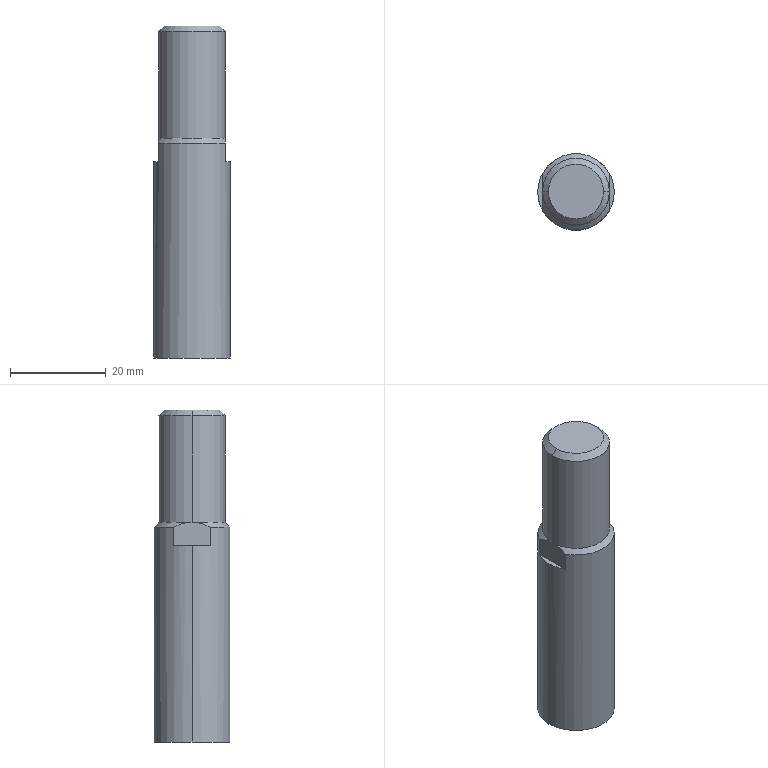Part | STEP file | rA_CDQ2B40_40DM_M9N_0_ | 1 solid | 14 faces | box 16 x 16 x 69.5 mm | volume 12766 mm3 | plane 6 | cylinder 4 | cone 4 | commonest cylinder face diameters 14 x2 16 x2
STEP:
#1=CARTESIAN_POINT('',(8.,0.,-41.));
#2=VERTEX_POINT('',#1);
#3=CARTESIAN_POINT('',(-8.,0.,-41.));
#4=VERTEX_POINT('',#3);
#5=CARTESIAN_POINT('',(0.,0.,-41.));
#6=DIRECTION('',(0.,0.,1.));
#7=DIRECTION('',(1.,0.,0.));
#8=AXIS2_PLACEMENT_3D('',#5,#6,#7);
#9=CIRCLE('',#8,8.);
#10=EDGE_CURVE('',#2,#4,#9,.T.);
#11=ORIENTED_EDGE('',*,*,#10,.T.);
#12=CARTESIAN_POINT('',(-8.,0.,0.1));
#13=VERTEX_POINT('',#12);
#14=CARTESIAN_POINT('',(-8.,0.,-41.));
#15=DIRECTION('',(0.,0.,1.));
#16=VECTOR('',#15,1000.);
#17=LINE('',#14,#16);
#18=EDGE_CURVE('',#4,#13,#17,.T.);
#19=ORIENTED_EDGE('',*,*,#18,.T.);
#20=CARTESIAN_POINT('',(-7.,3.873,0.1));
#21=VERTEX_POINT('',#20);
#22=CARTESIAN_POINT('',(0.,0.,0.1));
#23=DIRECTION('',(0.,0.,1.));
#24=DIRECTION('',(1.,0.,0.));
#25=AXIS2_PLACEMENT_3D('',#22,#23,#24);
#26=CIRCLE('',#25,8.);
#27=EDGE_CURVE('',#21,#13,#26,.T.);
#28=ORIENTED_EDGE('',*,*,#27,.F.);
#29=CARTESIAN_POINT('',(-7.,3.873,4.));
#30=VERTEX_POINT('',#29);
#31=CARTESIAN_POINT('',(-7.,3.873,-41.));
#32=DIRECTION('',(0.,0.,1.));
#33=VECTOR('',#32,1000.);
#34=LINE('',#31,#33);
#35=EDGE_CURVE('',#21,#30,#34,.T.);
#36=ORIENTED_EDGE('',*,*,#35,.T.);
#37=CARTESIAN_POINT('',(7.,3.873,4.));
#38=VERTEX_POINT('',#37);
#39=CARTESIAN_POINT('',(0.,0.,4.));
#40=DIRECTION('',(0.,0.,1.));
#41=DIRECTION('',(1.,0.,0.));
#42=AXIS2_PLACEMENT_3D('',#39,#40,#41);
#43=CIRCLE('',#42,8.);
#44=EDGE_CURVE('',#38,#30,#43,.T.);
#45=ORIENTED_EDGE('',*,*,#44,.F.);
#46=CARTESIAN_POINT('',(7.,3.873,0.1));
#47=VERTEX_POINT('',#46);
#48=CARTESIAN_POINT('',(7.,3.873,-41.));
#49=DIRECTION('',(0.,0.,-1.));
#50=VECTOR('',#49,1000.);
#51=LINE('',#48,#50);
#52=EDGE_CURVE('',#38,#47,#51,.T.);
#53=ORIENTED_EDGE('',*,*,#52,.T.);
#54=CARTESIAN_POINT('',(8.,0.,0.1));
#55=VERTEX_POINT('',#54);
#56=CARTESIAN_POINT('',(0.,0.,0.1));
#57=DIRECTION('',(0.,0.,1.));
#58=DIRECTION('',(1.,0.,0.));
#59=AXIS2_PLACEMENT_3D('',#56,#57,#58);
#60=CIRCLE('',#59,8.);
#61=EDGE_CURVE('',#55,#47,#60,.T.);
#62=ORIENTED_EDGE('',*,*,#61,.F.);
#63=CARTESIAN_POINT('',(8.,0.,-41.));
#64=DIRECTION('',(0.,0.,1.));
#65=VECTOR('',#64,1000.);
#66=LINE('',#63,#65);
#67=EDGE_CURVE('',#2,#55,#66,.T.);
#68=ORIENTED_EDGE('',*,*,#67,.F.);
#69=EDGE_LOOP('',(#11,#19,#28,#36,#45,#53,#62,#68));
#70=FACE_OUTER_BOUND('',#69,.T.);
#71=CARTESIAN_POINT('',(0.,0.,-41.));
#72=DIRECTION('',(0.,0.,1.));
#73=DIRECTION('',(1.,0.,0.));
#74=AXIS2_PLACEMENT_3D('',#71,#72,#73);
#75=CYLINDRICAL_SURFACE('',#74,8.);
#76=ADVANCED_FACE('',(#70),#75,.T.);
#77=CARTESIAN_POINT('',(7.,0.,5.));
#78=VERTEX_POINT('',#77);
#79=CARTESIAN_POINT('',(-7.,0.,5.));
#80=VERTEX_POINT('',#79);
#81=CARTESIAN_POINT('',(0.,0.,5.));
#82=DIRECTION('',(0.,0.,1.));
#83=DIRECTION('',(1.,0.,0.));
#84=AXIS2_PLACEMENT_3D('',#81,#82,#83);
#85=CIRCLE('',#84,7.);
#86=EDGE_CURVE('',#78,#80,#85,.T.);
#87=ORIENTED_EDGE('',*,*,#86,.T.);
#88=CARTESIAN_POINT('',(-7.,0.,27.275));
#89=VERTEX_POINT('',#88);
#90=CARTESIAN_POINT('',(-7.,0.,-41.));
#91=DIRECTION('',(0.,0.,1.));
#92=VECTOR('',#91,1000.);
#93=LINE('',#90,#92);
#94=EDGE_CURVE('',#80,#89,#93,.T.);
#95=ORIENTED_EDGE('',*,*,#94,.T.);
#96=CARTESIAN_POINT('',(7.,0.,27.275));
#97=VERTEX_POINT('',#96);
#98=CARTESIAN_POINT('',(0.,0.,27.275));
#99=DIRECTION('',(0.,0.,1.));
#100=DIRECTION('',(1.,0.,0.));
#101=AXIS2_PLACEMENT_3D('',#98,#99,#100);
#102=CIRCLE('',#101,7.);
#103=EDGE_CURVE('',#97,#89,#102,.T.);
#104=ORIENTED_EDGE('',*,*,#103,.F.);
#105=CARTESIAN_POINT('',(7.,0.,-41.));
#106=DIRECTION('',(0.,0.,1.));
#107=VECTOR('',#106,1000.);
#108=LINE('',#105,#107);
#109=EDGE_CURVE('',#78,#97,#108,.T.);
#110=ORIENTED_EDGE('',*,*,#109,.F.);
#111=EDGE_LOOP('',(#87,#95,#104,#110));
#112=FACE_OUTER_BOUND('',#111,.T.);
#113=CARTESIAN_POINT('',(0.,0.,-41.));
#114=DIRECTION('',(0.,0.,1.));
#115=DIRECTION('',(1.,0.,0.));
#116=AXIS2_PLACEMENT_3D('',#113,#114,#115);
#117=CYLINDRICAL_SURFACE('',#116,7.);
#118=ADVANCED_FACE('',(#112),#117,.T.);
#119=CARTESIAN_POINT('',(5.775,0.,28.5));
#120=VERTEX_POINT('',#119);
#121=CARTESIAN_POINT('',(-5.775,0.,28.5));
#122=VERTEX_POINT('',#121);
#123=CARTESIAN_POINT('',(0.,0.,28.5));
#124=DIRECTION('',(0.,0.,1.));
#125=DIRECTION('',(1.,0.,0.));
#126=AXIS2_PLACEMENT_3D('',#123,#124,#125);
#127=CIRCLE('',#126,5.775);
#128=EDGE_CURVE('',#120,#122,#127,.T.);
#129=ORIENTED_EDGE('',*,*,#128,.F.);
#130=CARTESIAN_POINT('',(7.,0.,27.275));
#131=DIRECTION('',(0.7071,0.,-0.7071));
#132=VECTOR('',#131,1000.);
#133=LINE('',#130,#132);
#134=EDGE_CURVE('',#120,#97,#133,.T.);
#135=ORIENTED_EDGE('',*,*,#134,.T.);
#136=ORIENTED_EDGE('',*,*,#103,.T.);
#137=CARTESIAN_POINT('',(-7.,0.,27.275));
#138=DIRECTION('',(-0.7071,0.,-0.7071));
#139=VECTOR('',#138,1000.);
#140=LINE('',#137,#139);
#141=EDGE_CURVE('',#122,#89,#140,.T.);
#142=ORIENTED_EDGE('',*,*,#141,.F.);
#143=EDGE_LOOP('',(#129,#135,#136,#142));
#144=FACE_OUTER_BOUND('',#143,.T.);
#145=CARTESIAN_POINT('',(0.,0.,27.275));
#146=DIRECTION('',(0.,0.,-1.));
#147=DIRECTION('',(-1.,0.,0.));
#148=AXIS2_PLACEMENT_3D('',#145,#146,#147);
#149=CONICAL_SURFACE('',#148,7.,0.7854);
#150=ADVANCED_FACE('',(#144),#149,.T.);
#151=CARTESIAN_POINT('',(-7.,-3.873,4.));
#152=VERTEX_POINT('',#151);
#153=CARTESIAN_POINT('',(7.,-3.873,4.));
#154=VERTEX_POINT('',#153);
#155=CARTESIAN_POINT('',(0.,0.,4.));
#156=DIRECTION('',(0.,0.,1.));
#157=DIRECTION('',(1.,0.,0.));
#158=AXIS2_PLACEMENT_3D('',#155,#156,#157);
#159=CIRCLE('',#158,8.);
#160=EDGE_CURVE('',#152,#154,#159,.T.);
#161=ORIENTED_EDGE('',*,*,#160,.T.);
#162=CARTESIAN_POINT('',(7.,-3.873,4.));
#163=CARTESIAN_POINT('',(7.,-3.276,4.289));
#164=CARTESIAN_POINT('',(7.,-2.656,4.54));
#165=CARTESIAN_POINT('',(7.,-1.346,4.9));
#166=CARTESIAN_POINT('',(7.,-0.6799,5.));
#167=CARTESIAN_POINT('',(7.,0.,5.));
#168=B_SPLINE_CURVE_WITH_KNOTS('',3,(#162,#163,#164,#165,#166,#167),.UNSPECIFIED.,.F.,.F.,(4,2,4),(0.02013,0.02213,0.02413),.UNSPECIFIED.);
#169=EDGE_CURVE('',#154,#78,#168,.T.);
#170=ORIENTED_EDGE('',*,*,#169,.T.);
#171=CARTESIAN_POINT('',(0.,0.,5.));
#172=DIRECTION('',(0.,0.,1.));
#173=DIRECTION('',(1.,0.,0.));
#174=AXIS2_PLACEMENT_3D('',#171,#172,#173);
#175=CIRCLE('',#174,7.);
#176=EDGE_CURVE('',#80,#78,#175,.T.);
#177=ORIENTED_EDGE('',*,*,#176,.F.);
#178=CARTESIAN_POINT('',(-7.,0.,5.));
#179=CARTESIAN_POINT('',(-7.,-0.6799,5.));
#180=CARTESIAN_POINT('',(-7.,-1.346,4.9));
#181=CARTESIAN_POINT('',(-7.,-2.656,4.54));
#182=CARTESIAN_POINT('',(-7.,-3.276,4.289));
#183=CARTESIAN_POINT('',(-7.,-3.873,4.));
#184=B_SPLINE_CURVE_WITH_KNOTS('',3,(#178,#179,#180,#181,#182,#183),.UNSPECIFIED.,.F.,.F.,(4,2,4),(0.008364,0.01037,0.01237),.UNSPECIFIED.);
#185=EDGE_CURVE('',#80,#152,#184,.T.);
#186=ORIENTED_EDGE('',*,*,#185,.T.);
#187=EDGE_LOOP('',(#161,#170,#177,#186));
#188=FACE_OUTER_BOUND('',#187,.T.);
#189=CARTESIAN_POINT('',(0.,0.,4.));
#190=DIRECTION('',(0.,0.,-1.));
#191=DIRECTION('',(-1.,0.,0.));
#192=AXIS2_PLACEMENT_3D('',#189,#190,#191);
#193=CONICAL_SURFACE('',#192,8.,0.7854);
#194=ADVANCED_FACE('',(#188),#193,.T.);
#195=CARTESIAN_POINT('',(0.,0.,28.5));
#196=DIRECTION('',(0.,0.,1.));
#197=DIRECTION('',(1.,0.,0.));
#198=AXIS2_PLACEMENT_3D('',#195,#196,#197);
#199=CIRCLE('',#198,5.775);
#200=EDGE_CURVE('',#122,#120,#199,.T.);
#201=ORIENTED_EDGE('',*,*,#200,.T.);
#202=ORIENTED_EDGE('',*,*,#128,.T.);
#203=EDGE_LOOP('',(#201,#202));
#204=FACE_OUTER_BOUND('',#203,.T.);
#205=CARTESIAN_POINT('',(0.,0.,28.5));
#206=DIRECTION('',(0.,0.,-1.));
#207=DIRECTION('',(-1.,0.,0.));
#208=AXIS2_PLACEMENT_3D('',#205,#206,#207);
#209=PLANE('',#208);
#210=ADVANCED_FACE('',(#204),#209,.F.);
#211=ORIENTED_EDGE('',*,*,#134,.F.);
#212=ORIENTED_EDGE('',*,*,#200,.F.);
#213=ORIENTED_EDGE('',*,*,#141,.T.);
#214=CARTESIAN_POINT('',(0.,0.,27.275));
#215=DIRECTION('',(0.,0.,1.));
#216=DIRECTION('',(1.,0.,0.));
#217=AXIS2_PLACEMENT_3D('',#214,#215,#216);
#218=CIRCLE('',#217,7.);
#219=EDGE_CURVE('',#89,#97,#218,.T.);
#220=ORIENTED_EDGE('',*,*,#219,.T.);
#221=EDGE_LOOP('',(#211,#212,#213,#220));
#222=FACE_OUTER_BOUND('',#221,.T.);
#223=CARTESIAN_POINT('',(0.,0.,27.275));
#224=DIRECTION('',(0.,0.,-1.));
#225=DIRECTION('',(-1.,0.,0.));
#226=AXIS2_PLACEMENT_3D('',#223,#224,#225);
#227=CONICAL_SURFACE('',#226,7.,0.7854);
#228=ADVANCED_FACE('',(#222),#227,.T.);
#229=ORIENTED_EDGE('',*,*,#94,.F.);
#230=ORIENTED_EDGE('',*,*,#176,.T.);
#231=ORIENTED_EDGE('',*,*,#109,.T.);
#232=ORIENTED_EDGE('',*,*,#219,.F.);
#233=EDGE_LOOP('',(#229,#230,#231,#232));
#234=FACE_OUTER_BOUND('',#233,.T.);
#235=CARTESIAN_POINT('',(0.,0.,-41.));
#236=DIRECTION('',(0.,0.,1.));
#237=DIRECTION('',(1.,0.,0.));
#238=AXIS2_PLACEMENT_3D('',#235,#236,#237);
#239=CYLINDRICAL_SURFACE('',#238,7.);
#240=ADVANCED_FACE('',(#234),#239,.T.);
#241=ORIENTED_EDGE('',*,*,#86,.F.);
#242=CARTESIAN_POINT('',(7.,0.,5.));
#243=CARTESIAN_POINT('',(7.,0.3393,5.));
#244=CARTESIAN_POINT('',(7.,0.6764,4.975));
#245=CARTESIAN_POINT('',(7.,1.34,4.88));
#246=CARTESIAN_POINT('',(7.,1.668,4.811));
#247=CARTESIAN_POINT('',(7.,2.316,4.633));
#248=CARTESIAN_POINT('',(7.,2.639,4.525));
#249=CARTESIAN_POINT('',(7.,3.266,4.281));
#250=CARTESIAN_POINT('',(7.,3.573,4.145));
#251=CARTESIAN_POINT('',(7.,3.873,4.));
#252=B_SPLINE_CURVE_WITH_KNOTS('',3,(#242,#243,#244,#245,#246,#247,#248,#249,#250,#251),.UNSPECIFIED.,.F.,.F.,(4,2,2,2,4),(0.02413,0.02513,0.02612,0.02712,0.02812),.UNSPECIFIED.);
#253=EDGE_CURVE('',#78,#38,#252,.T.);
#254=ORIENTED_EDGE('',*,*,#253,.T.);
#255=ORIENTED_EDGE('',*,*,#44,.T.);
#256=CARTESIAN_POINT('',(-7.,3.873,4.));
#257=CARTESIAN_POINT('',(-7.,3.573,4.145));
#258=CARTESIAN_POINT('',(-7.,3.266,4.281));
#259=CARTESIAN_POINT('',(-7.,2.639,4.525));
#260=CARTESIAN_POINT('',(-7.,2.316,4.633));
#261=CARTESIAN_POINT('',(-7.,1.668,4.811));
#262=CARTESIAN_POINT('',(-7.,1.34,4.88));
#263=CARTESIAN_POINT('',(-7.,0.6764,4.975));
#264=CARTESIAN_POINT('',(-7.,0.3393,5.));
#265=CARTESIAN_POINT('',(-7.,0.,5.));
#266=B_SPLINE_CURVE_WITH_KNOTS('',3,(#256,#257,#258,#259,#260,#261,#262,#263,#264,#265),.UNSPECIFIED.,.F.,.F.,(4,2,2,2,4),(0.004369,0.005367,0.006366,0.007365,0.008364),.UNSPECIFIED.);
#267=EDGE_CURVE('',#30,#80,#266,.T.);
#268=ORIENTED_EDGE('',*,*,#267,.T.);
#269=EDGE_LOOP('',(#241,#254,#255,#268));
#270=FACE_OUTER_BOUND('',#269,.T.);
#271=CARTESIAN_POINT('',(0.,0.,4.));
#272=DIRECTION('',(0.,0.,-1.));
#273=DIRECTION('',(-1.,0.,0.));
#274=AXIS2_PLACEMENT_3D('',#271,#272,#273);
#275=CONICAL_SURFACE('',#274,8.,0.7854);
#276=ADVANCED_FACE('',(#270),#275,.T.);
#277=ORIENTED_EDGE('',*,*,#18,.F.);
#278=CARTESIAN_POINT('',(0.,0.,-41.));
#279=DIRECTION('',(0.,0.,1.));
#280=DIRECTION('',(1.,0.,0.));
#281=AXIS2_PLACEMENT_3D('',#278,#279,#280);
#282=CIRCLE('',#281,8.);
#283=EDGE_CURVE('',#4,#2,#282,.T.);
#284=ORIENTED_EDGE('',*,*,#283,.T.);
#285=ORIENTED_EDGE('',*,*,#67,.T.);
#286=CARTESIAN_POINT('',(7.,-3.873,0.1));
#287=VERTEX_POINT('',#286);
#288=CARTESIAN_POINT('',(0.,0.,0.1));
#289=DIRECTION('',(0.,0.,1.));
#290=DIRECTION('',(1.,0.,0.));
#291=AXIS2_PLACEMENT_3D('',#288,#289,#290);
#292=CIRCLE('',#291,8.);
#293=EDGE_CURVE('',#287,#55,#292,.T.);
#294=ORIENTED_EDGE('',*,*,#293,.F.);
#295=CARTESIAN_POINT('',(7.,-3.873,-41.));
#296=DIRECTION('',(0.,0.,1.));
#297=VECTOR('',#296,1000.);
#298=LINE('',#295,#297);
#299=EDGE_CURVE('',#287,#154,#298,.T.);
#300=ORIENTED_EDGE('',*,*,#299,.T.);
#301=ORIENTED_EDGE('',*,*,#160,.F.);
#302=CARTESIAN_POINT('',(-7.,-3.873,0.1));
#303=VERTEX_POINT('',#302);
#304=CARTESIAN_POINT('',(-7.,-3.873,-41.));
#305=DIRECTION('',(0.,0.,-1.));
#306=VECTOR('',#305,1000.);
#307=LINE('',#304,#306);
#308=EDGE_CURVE('',#152,#303,#307,.T.);
#309=ORIENTED_EDGE('',*,*,#308,.T.);
#310=CARTESIAN_POINT('',(0.,0.,0.1));
#311=DIRECTION('',(0.,0.,1.));
#312=DIRECTION('',(1.,0.,0.));
#313=AXIS2_PLACEMENT_3D('',#310,#311,#312);
#314=CIRCLE('',#313,8.);
#315=EDGE_CURVE('',#13,#303,#314,.T.);
#316=ORIENTED_EDGE('',*,*,#315,.F.);
#317=EDGE_LOOP('',(#277,#284,#285,#294,#300,#301,#309,#316));
#318=FACE_OUTER_BOUND('',#317,.T.);
#319=CARTESIAN_POINT('',(0.,0.,-41.));
#320=DIRECTION('',(0.,0.,1.));
#321=DIRECTION('',(1.,0.,0.));
#322=AXIS2_PLACEMENT_3D('',#319,#320,#321);
#323=CYLINDRICAL_SURFACE('',#322,8.);
#324=ADVANCED_FACE('',(#318),#323,.T.);
#325=ORIENTED_EDGE('',*,*,#10,.F.);
#326=ORIENTED_EDGE('',*,*,#283,.F.);
#327=EDGE_LOOP('',(#325,#326));
#328=FACE_OUTER_BOUND('',#327,.T.);
#329=CARTESIAN_POINT('',(0.,8.,-41.));
#330=DIRECTION('',(0.,0.,1.));
#331=DIRECTION('',(1.,0.,0.));
#332=AXIS2_PLACEMENT_3D('',#329,#330,#331);
#333=PLANE('',#332);
#334=ADVANCED_FACE('',(#328),#333,.F.);
#335=ORIENTED_EDGE('',*,*,#293,.T.);
#336=ORIENTED_EDGE('',*,*,#61,.T.);
#337=CARTESIAN_POINT('',(7.,10.,0.1));
#338=DIRECTION('',(0.,-1.,0.));
#339=VECTOR('',#338,1000.);
#340=LINE('',#337,#339);
#341=EDGE_CURVE('',#47,#287,#340,.T.);
#342=ORIENTED_EDGE('',*,*,#341,.T.);
#343=EDGE_LOOP('',(#335,#336,#342));
#344=FACE_OUTER_BOUND('',#343,.T.);
#345=CARTESIAN_POINT('',(-10.,-10.,0.1));
#346=DIRECTION('',(0.,0.,1.));
#347=DIRECTION('',(1.,0.,0.));
#348=AXIS2_PLACEMENT_3D('',#345,#346,#347);
#349=PLANE('',#348);
#350=ADVANCED_FACE('',(#344),#349,.T.);
#351=ORIENTED_EDGE('',*,*,#341,.F.);
#352=ORIENTED_EDGE('',*,*,#52,.F.);
#353=ORIENTED_EDGE('',*,*,#253,.F.);
#354=ORIENTED_EDGE('',*,*,#169,.F.);
#355=ORIENTED_EDGE('',*,*,#299,.F.);
#356=EDGE_LOOP('',(#351,#352,#353,#354,#355));
#357=FACE_OUTER_BOUND('',#356,.T.);
#358=CARTESIAN_POINT('',(7.,10.,0.1));
#359=DIRECTION('',(-1.,0.,0.));
#360=DIRECTION('',(0.,0.,1.));
#361=AXIS2_PLACEMENT_3D('',#358,#359,#360);
#362=PLANE('',#361);
#363=ADVANCED_FACE('',(#357),#362,.F.);
#364=CARTESIAN_POINT('',(-7.,-10.,0.1));
#365=DIRECTION('',(0.,1.,0.));
#366=VECTOR('',#365,1000.);
#367=LINE('',#364,#366);
#368=EDGE_CURVE('',#303,#21,#367,.T.);
#369=ORIENTED_EDGE('',*,*,#368,.F.);
#370=ORIENTED_EDGE('',*,*,#308,.F.);
#371=ORIENTED_EDGE('',*,*,#185,.F.);
#372=ORIENTED_EDGE('',*,*,#267,.F.);
#373=ORIENTED_EDGE('',*,*,#35,.F.);
#374=EDGE_LOOP('',(#369,#370,#371,#372,#373));
#375=FACE_OUTER_BOUND('',#374,.T.);
#376=CARTESIAN_POINT('',(-7.,-10.,0.1));
#377=DIRECTION('',(1.,0.,0.));
#378=DIRECTION('',(0.,0.,-1.));
#379=AXIS2_PLACEMENT_3D('',#376,#377,#378);
#380=PLANE('',#379);
#381=ADVANCED_FACE('',(#375),#380,.F.);
#382=ORIENTED_EDGE('',*,*,#27,.T.);
#383=ORIENTED_EDGE('',*,*,#315,.T.);
#384=ORIENTED_EDGE('',*,*,#368,.T.);
#385=EDGE_LOOP('',(#382,#383,#384));
#386=FACE_OUTER_BOUND('',#385,.T.);
#387=CARTESIAN_POINT('',(-10.,-10.,0.1));
#388=DIRECTION('',(0.,0.,1.));
#389=DIRECTION('',(1.,0.,0.));
#390=AXIS2_PLACEMENT_3D('',#387,#388,#389);
#391=PLANE('',#390);
#392=ADVANCED_FACE('',(#386),#391,.T.);
#393=CLOSED_SHELL('',(#76,#118,#150,#194,#210,#228,#240,#276,#324,#334,#350,#363,#381,#392));
#394=MANIFOLD_SOLID_BREP('',#393);
#395=CARTESIAN_POINT('',(0.,0.,0.));
#396=DIRECTION('',(0.,0.,1.));
#397=DIRECTION('',(1.,0.,0.));
#398=AXIS2_PLACEMENT_3D('',#395,#396,#397);
#399=(LENGTH_UNIT()NAMED_UNIT(*)SI_UNIT(.MILLI.,.METRE.));
#400=UNCERTAINTY_MEASURE_WITH_UNIT(LENGTH_MEASURE(0.00001),#399,'','');
#401=(NAMED_UNIT(*)PLANE_ANGLE_UNIT()SI_UNIT($,.RADIAN.));
#402=(NAMED_UNIT(*)SI_UNIT($,.STERADIAN.)SOLID_ANGLE_UNIT());
#403=(GEOMETRIC_REPRESENTATION_CONTEXT(3)GLOBAL_UNCERTAINTY_ASSIGNED_CONTEXT((#400))GLOBAL_UNIT_ASSIGNED_CONTEXT((#399,#401,#402))REPRESENTATION_CONTEXT('',''));
#404=ADVANCED_BREP_SHAPE_REPRESENTATION('',(#394,#398),#403);